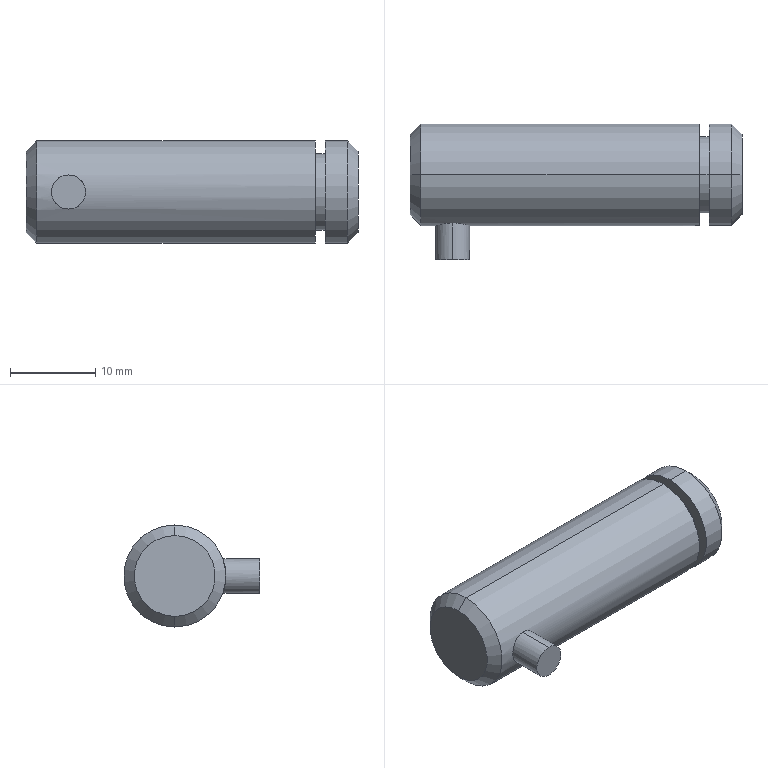Part | SolidWorks | features Revolution 2, Chamfer 1 | 1 solid | 17 faces | box 39 x 16 x 12 mm | volume 4350 mm3 | cylinder 8 | plane 5 | cone 4 | commonest cylinder face diameters 12 x4 4 x2 9 x2
STEP:
#1=CARTESIAN_POINT('',(19.5,0.,-4.75));
#2=VERTEX_POINT('',#1);
#3=CARTESIAN_POINT('',(19.5,0.,4.75));
#4=VERTEX_POINT('',#3);
#5=CARTESIAN_POINT('',(19.5,0.,0.));
#6=DIRECTION('',(1.,0.,0.));
#7=DIRECTION('',(0.,0.,-1.));
#8=AXIS2_PLACEMENT_3D('',#5,#6,#7);
#9=CIRCLE('',#8,4.75);
#10=EDGE_CURVE('',#2,#4,#9,.T.);
#11=ORIENTED_EDGE('',*,*,#10,.F.);
#12=CARTESIAN_POINT('',(18.25,0.,-6.));
#13=VERTEX_POINT('',#12);
#14=CARTESIAN_POINT('',(18.25,0.,-6.));
#15=DIRECTION('',(-0.7071,0.,-0.7071));
#16=VECTOR('',#15,1000.);
#17=LINE('',#14,#16);
#18=EDGE_CURVE('',#2,#13,#17,.T.);
#19=ORIENTED_EDGE('',*,*,#18,.T.);
#20=CARTESIAN_POINT('',(18.25,0.,6.));
#21=VERTEX_POINT('',#20);
#22=CARTESIAN_POINT('',(18.25,0.,0.));
#23=DIRECTION('',(-1.,0.,0.));
#24=DIRECTION('',(0.,0.,-1.));
#25=AXIS2_PLACEMENT_3D('',#22,#23,#24);
#26=CIRCLE('',#25,6.);
#27=EDGE_CURVE('',#21,#13,#26,.T.);
#28=ORIENTED_EDGE('',*,*,#27,.F.);
#29=CARTESIAN_POINT('',(18.25,0.,6.));
#30=DIRECTION('',(-0.7071,0.,0.7071));
#31=VECTOR('',#30,1000.);
#32=LINE('',#29,#31);
#33=EDGE_CURVE('',#4,#21,#32,.T.);
#34=ORIENTED_EDGE('',*,*,#33,.F.);
#35=EDGE_LOOP('',(#11,#19,#28,#34));
#36=FACE_OUTER_BOUND('',#35,.T.);
#37=CARTESIAN_POINT('',(18.25,0.,0.));
#38=DIRECTION('',(-1.,0.,0.));
#39=DIRECTION('',(0.,0.,1.));
#40=AXIS2_PLACEMENT_3D('',#37,#38,#39);
#41=CONICAL_SURFACE('',#40,6.,0.7854);
#42=ADVANCED_FACE('',(#36),#41,.T.);
#43=CARTESIAN_POINT('',(-19.5,0.,4.75));
#44=VERTEX_POINT('',#43);
#45=CARTESIAN_POINT('',(-19.5,0.,-4.75));
#46=VERTEX_POINT('',#45);
#47=CARTESIAN_POINT('',(-19.5,0.,0.));
#48=DIRECTION('',(-1.,0.,0.));
#49=DIRECTION('',(0.,0.,1.));
#50=AXIS2_PLACEMENT_3D('',#47,#48,#49);
#51=CIRCLE('',#50,4.75);
#52=EDGE_CURVE('',#44,#46,#51,.T.);
#53=ORIENTED_EDGE('',*,*,#52,.F.);
#54=CARTESIAN_POINT('',(-18.25,0.,6.));
#55=VERTEX_POINT('',#54);
#56=CARTESIAN_POINT('',(-19.5,0.,4.75));
#57=DIRECTION('',(0.7071,0.,0.7071));
#58=VECTOR('',#57,1000.);
#59=LINE('',#56,#58);
#60=EDGE_CURVE('',#44,#55,#59,.T.);
#61=ORIENTED_EDGE('',*,*,#60,.T.);
#62=CARTESIAN_POINT('',(-18.25,0.,-6.));
#63=VERTEX_POINT('',#62);
#64=CARTESIAN_POINT('',(-18.25,0.,0.));
#65=DIRECTION('',(1.,0.,0.));
#66=DIRECTION('',(0.,0.,1.));
#67=AXIS2_PLACEMENT_3D('',#64,#65,#66);
#68=CIRCLE('',#67,6.);
#69=EDGE_CURVE('',#63,#55,#68,.T.);
#70=ORIENTED_EDGE('',*,*,#69,.F.);
#71=CARTESIAN_POINT('',(-19.5,0.,-4.75));
#72=DIRECTION('',(0.7071,0.,-0.7071));
#73=VECTOR('',#72,1000.);
#74=LINE('',#71,#73);
#75=EDGE_CURVE('',#46,#63,#74,.T.);
#76=ORIENTED_EDGE('',*,*,#75,.F.);
#77=EDGE_LOOP('',(#53,#61,#70,#76));
#78=FACE_OUTER_BOUND('',#77,.T.);
#79=CARTESIAN_POINT('',(-19.5,0.,0.));
#80=DIRECTION('',(1.,0.,0.));
#81=DIRECTION('',(0.,0.,-1.));
#82=AXIS2_PLACEMENT_3D('',#79,#80,#81);
#83=CONICAL_SURFACE('',#82,4.75,0.7854);
#84=ADVANCED_FACE('',(#78),#83,.T.);
#85=CARTESIAN_POINT('',(-14.5,-5.657,-2.));
#86=VERTEX_POINT('',#85);
#87=CARTESIAN_POINT('',(-14.5,-5.657,2.));
#88=VERTEX_POINT('',#87);
#89=CARTESIAN_POINT('',(-14.5,-5.657,-2.));
#90=CARTESIAN_POINT('',(-14.367,-5.657,-2.));
#91=CARTESIAN_POINT('',(-14.236,-5.662,-1.987));
#92=CARTESIAN_POINT('',(-13.979,-5.679,-1.935));
#93=CARTESIAN_POINT('',(-13.852,-5.693,-1.897));
#94=CARTESIAN_POINT('',(-13.61,-5.725,-1.796));
#95=CARTESIAN_POINT('',(-13.495,-5.744,-1.734));
#96=CARTESIAN_POINT('',(-13.279,-5.786,-1.589));
#97=CARTESIAN_POINT('',(-13.177,-5.809,-1.506));
#98=CARTESIAN_POINT('',(-12.902,-5.875,-1.231));
#99=CARTESIAN_POINT('',(-12.754,-5.919,-1.009));
#100=CARTESIAN_POINT('',(-12.604,-5.966,-0.6487));
#101=CARTESIAN_POINT('',(-12.565,-5.979,-0.5216));
#102=CARTESIAN_POINT('',(-12.513,-5.996,-0.2629));
#103=CARTESIAN_POINT('',(-12.5,-6.,-0.1325));
#104=CARTESIAN_POINT('',(-12.5,-6.,0.1306));
#105=CARTESIAN_POINT('',(-12.513,-5.996,0.2642));
#106=CARTESIAN_POINT('',(-12.565,-5.979,0.5216));
#107=CARTESIAN_POINT('',(-12.603,-5.966,0.6468));
#108=CARTESIAN_POINT('',(-12.704,-5.935,0.8903));
#109=CARTESIAN_POINT('',(-12.766,-5.916,1.006));
#110=CARTESIAN_POINT('',(-12.911,-5.875,1.221));
#111=CARTESIAN_POINT('',(-12.995,-5.853,1.323));
#112=CARTESIAN_POINT('',(-13.179,-5.808,1.507));
#113=CARTESIAN_POINT('',(-13.279,-5.786,1.589));
#114=CARTESIAN_POINT('',(-13.495,-5.744,1.734));
#115=CARTESIAN_POINT('',(-13.612,-5.725,1.797));
#116=CARTESIAN_POINT('',(-13.853,-5.693,1.897));
#117=CARTESIAN_POINT('',(-13.977,-5.679,1.935));
#118=CARTESIAN_POINT('',(-14.236,-5.662,1.987));
#119=CARTESIAN_POINT('',(-14.369,-5.657,2.));
#120=CARTESIAN_POINT('',(-14.5,-5.657,2.));
#121=B_SPLINE_CURVE_WITH_KNOTS('',3,(#89,#90,#91,#92,#93,#94,#95,#96,#97,#98,#99,#100,#101,#102,#103,#104,#105,#106,#107,#108,#109,#110,#111,#112,#113,#114,#115,#116,#117,#118,#119,#120),.UNSPECIFIED.,.F.,.F.,(4,2,2,2,2,2,2,2,2,2,2,2,2,2,2,4),(0.,0.0003936,0.0007873,0.001181,0.001575,0.002362,0.002755,0.003149,0.003543,0.003936,0.00433,0.004724,0.005117,0.005511,0.005905,0.006298),.UNSPECIFIED.);
#122=EDGE_CURVE('',#86,#88,#121,.T.);
#123=ORIENTED_EDGE('',*,*,#122,.T.);
#124=CARTESIAN_POINT('',(-14.5,-10.,2.));
#125=VERTEX_POINT('',#124);
#126=CARTESIAN_POINT('',(-14.5,-5.657,2.));
#127=DIRECTION('',(0.,-1.,0.));
#128=VECTOR('',#127,1000.);
#129=LINE('',#126,#128);
#130=EDGE_CURVE('',#88,#125,#129,.T.);
#131=ORIENTED_EDGE('',*,*,#130,.T.);
#132=CARTESIAN_POINT('',(-14.5,-10.,-2.));
#133=VERTEX_POINT('',#132);
#134=CARTESIAN_POINT('',(-14.5,-10.,0.));
#135=DIRECTION('',(0.,-1.,0.));
#136=DIRECTION('',(0.,0.,-1.));
#137=AXIS2_PLACEMENT_3D('',#134,#135,#136);
#138=CIRCLE('',#137,2.);
#139=EDGE_CURVE('',#133,#125,#138,.T.);
#140=ORIENTED_EDGE('',*,*,#139,.F.);
#141=CARTESIAN_POINT('',(-14.5,-5.657,-2.));
#142=DIRECTION('',(0.,-1.,0.));
#143=VECTOR('',#142,1000.);
#144=LINE('',#141,#143);
#145=EDGE_CURVE('',#86,#133,#144,.T.);
#146=ORIENTED_EDGE('',*,*,#145,.F.);
#147=EDGE_LOOP('',(#123,#131,#140,#146));
#148=FACE_OUTER_BOUND('',#147,.T.);
#149=CARTESIAN_POINT('',(-14.5,-5.657,0.));
#150=DIRECTION('',(0.,-1.,0.));
#151=DIRECTION('',(0.,0.,-1.));
#152=AXIS2_PLACEMENT_3D('',#149,#150,#151);
#153=CYLINDRICAL_SURFACE('',#152,2.);
#154=ADVANCED_FACE('',(#148),#153,.T.);
#155=CARTESIAN_POINT('',(15.65,0.,4.5));
#156=VERTEX_POINT('',#155);
#157=CARTESIAN_POINT('',(15.65,0.,-4.5));
#158=VERTEX_POINT('',#157);
#159=CARTESIAN_POINT('',(15.65,0.,0.));
#160=DIRECTION('',(-1.,0.,0.));
#161=DIRECTION('',(0.,0.,1.));
#162=AXIS2_PLACEMENT_3D('',#159,#160,#161);
#163=CIRCLE('',#162,4.5);
#164=EDGE_CURVE('',#156,#158,#163,.T.);
#165=ORIENTED_EDGE('',*,*,#164,.T.);
#166=CARTESIAN_POINT('',(14.5,0.,-4.5));
#167=VERTEX_POINT('',#166);
#168=CARTESIAN_POINT('',(19.5,0.,-4.5));
#169=DIRECTION('',(-1.,0.,0.));
#170=VECTOR('',#169,1000.);
#171=LINE('',#168,#170);
#172=EDGE_CURVE('',#158,#167,#171,.T.);
#173=ORIENTED_EDGE('',*,*,#172,.T.);
#174=CARTESIAN_POINT('',(14.5,0.,4.5));
#175=VERTEX_POINT('',#174);
#176=CARTESIAN_POINT('',(14.5,0.,0.));
#177=DIRECTION('',(-1.,0.,0.));
#178=DIRECTION('',(0.,0.,1.));
#179=AXIS2_PLACEMENT_3D('',#176,#177,#178);
#180=CIRCLE('',#179,4.5);
#181=EDGE_CURVE('',#175,#167,#180,.T.);
#182=ORIENTED_EDGE('',*,*,#181,.F.);
#183=CARTESIAN_POINT('',(19.5,0.,4.5));
#184=DIRECTION('',(-1.,0.,0.));
#185=VECTOR('',#184,1000.);
#186=LINE('',#183,#185);
#187=EDGE_CURVE('',#156,#175,#186,.T.);
#188=ORIENTED_EDGE('',*,*,#187,.F.);
#189=EDGE_LOOP('',(#165,#173,#182,#188));
#190=FACE_OUTER_BOUND('',#189,.T.);
#191=CARTESIAN_POINT('',(19.5,0.,0.));
#192=DIRECTION('',(-1.,0.,0.));
#193=DIRECTION('',(0.,0.,1.));
#194=AXIS2_PLACEMENT_3D('',#191,#192,#193);
#195=CYLINDRICAL_SURFACE('',#194,4.5);
#196=ADVANCED_FACE('',(#190),#195,.T.);
#197=CARTESIAN_POINT('',(14.5,0.,6.));
#198=VERTEX_POINT('',#197);
#199=CARTESIAN_POINT('',(14.5,0.,-6.));
#200=VERTEX_POINT('',#199);
#201=CARTESIAN_POINT('',(14.5,0.,0.));
#202=DIRECTION('',(-1.,0.,0.));
#203=DIRECTION('',(0.,0.,1.));
#204=AXIS2_PLACEMENT_3D('',#201,#202,#203);
#205=CIRCLE('',#204,6.);
#206=EDGE_CURVE('',#198,#200,#205,.T.);
#207=ORIENTED_EDGE('',*,*,#206,.T.);
#208=CARTESIAN_POINT('',(19.5,0.,-6.));
#209=DIRECTION('',(-1.,0.,0.));
#210=VECTOR('',#209,1000.);
#211=LINE('',#208,#210);
#212=EDGE_CURVE('',#200,#63,#211,.T.);
#213=ORIENTED_EDGE('',*,*,#212,.T.);
#214=ORIENTED_EDGE('',*,*,#69,.T.);
#215=CARTESIAN_POINT('',(19.5,0.,6.));
#216=DIRECTION('',(-1.,0.,0.));
#217=VECTOR('',#216,1000.);
#218=LINE('',#215,#217);
#219=EDGE_CURVE('',#198,#55,#218,.T.);
#220=ORIENTED_EDGE('',*,*,#219,.F.);
#221=EDGE_LOOP('',(#207,#213,#214,#220));
#222=FACE_OUTER_BOUND('',#221,.T.);
#223=CARTESIAN_POINT('',(19.5,0.,0.));
#224=DIRECTION('',(-1.,0.,0.));
#225=DIRECTION('',(0.,0.,1.));
#226=AXIS2_PLACEMENT_3D('',#223,#224,#225);
#227=CYLINDRICAL_SURFACE('',#226,6.);
#228=ADVANCED_FACE('',(#222),#227,.T.);
#229=ORIENTED_EDGE('',*,*,#27,.T.);
#230=CARTESIAN_POINT('',(15.65,0.,-6.));
#231=VERTEX_POINT('',#230);
#232=CARTESIAN_POINT('',(19.5,0.,-6.));
#233=DIRECTION('',(-1.,0.,0.));
#234=VECTOR('',#233,1000.);
#235=LINE('',#232,#234);
#236=EDGE_CURVE('',#13,#231,#235,.T.);
#237=ORIENTED_EDGE('',*,*,#236,.T.);
#238=CARTESIAN_POINT('',(15.65,0.,6.));
#239=VERTEX_POINT('',#238);
#240=CARTESIAN_POINT('',(15.65,0.,0.));
#241=DIRECTION('',(-1.,0.,0.));
#242=DIRECTION('',(0.,0.,1.));
#243=AXIS2_PLACEMENT_3D('',#240,#241,#242);
#244=CIRCLE('',#243,6.);
#245=EDGE_CURVE('',#239,#231,#244,.T.);
#246=ORIENTED_EDGE('',*,*,#245,.F.);
#247=CARTESIAN_POINT('',(19.5,0.,6.));
#248=DIRECTION('',(-1.,0.,0.));
#249=VECTOR('',#248,1000.);
#250=LINE('',#247,#249);
#251=EDGE_CURVE('',#21,#239,#250,.T.);
#252=ORIENTED_EDGE('',*,*,#251,.F.);
#253=EDGE_LOOP('',(#229,#237,#246,#252));
#254=FACE_OUTER_BOUND('',#253,.T.);
#255=CARTESIAN_POINT('',(19.5,0.,0.));
#256=DIRECTION('',(-1.,0.,0.));
#257=DIRECTION('',(0.,0.,1.));
#258=AXIS2_PLACEMENT_3D('',#255,#256,#257);
#259=CYLINDRICAL_SURFACE('',#258,6.);
#260=ADVANCED_FACE('',(#254),#259,.T.);
#261=ORIENTED_EDGE('',*,*,#236,.F.);
#262=CARTESIAN_POINT('',(18.25,0.,0.));
#263=DIRECTION('',(-1.,0.,0.));
#264=DIRECTION('',(0.,0.,-1.));
#265=AXIS2_PLACEMENT_3D('',#262,#263,#264);
#266=CIRCLE('',#265,6.);
#267=EDGE_CURVE('',#13,#21,#266,.T.);
#268=ORIENTED_EDGE('',*,*,#267,.T.);
#269=ORIENTED_EDGE('',*,*,#251,.T.);
#270=CARTESIAN_POINT('',(15.65,0.,0.));
#271=DIRECTION('',(-1.,0.,0.));
#272=DIRECTION('',(0.,0.,1.));
#273=AXIS2_PLACEMENT_3D('',#270,#271,#272);
#274=CIRCLE('',#273,6.);
#275=EDGE_CURVE('',#231,#239,#274,.T.);
#276=ORIENTED_EDGE('',*,*,#275,.F.);
#277=EDGE_LOOP('',(#261,#268,#269,#276));
#278=FACE_OUTER_BOUND('',#277,.T.);
#279=CARTESIAN_POINT('',(19.5,0.,0.));
#280=DIRECTION('',(-1.,0.,0.));
#281=DIRECTION('',(0.,0.,1.));
#282=AXIS2_PLACEMENT_3D('',#279,#280,#281);
#283=CYLINDRICAL_SURFACE('',#282,6.);
#284=ADVANCED_FACE('',(#278),#283,.T.);
#285=CARTESIAN_POINT('',(19.5,0.,0.));
#286=DIRECTION('',(1.,0.,0.));
#287=DIRECTION('',(0.,0.,-1.));
#288=AXIS2_PLACEMENT_3D('',#285,#286,#287);
#289=CIRCLE('',#288,4.75);
#290=EDGE_CURVE('',#4,#2,#289,.T.);
#291=ORIENTED_EDGE('',*,*,#290,.T.);
#292=ORIENTED_EDGE('',*,*,#10,.T.);
#293=EDGE_LOOP('',(#291,#292));
#294=FACE_OUTER_BOUND('',#293,.T.);
#295=CARTESIAN_POINT('',(19.5,6.,0.));
#296=DIRECTION('',(1.,0.,0.));
#297=DIRECTION('',(0.,0.,-1.));
#298=AXIS2_PLACEMENT_3D('',#295,#296,#297);
#299=PLANE('',#298);
#300=ADVANCED_FACE('',(#294),#299,.T.);
#301=CARTESIAN_POINT('',(-19.5,0.,0.));
#302=DIRECTION('',(-1.,0.,0.));
#303=DIRECTION('',(0.,0.,1.));
#304=AXIS2_PLACEMENT_3D('',#301,#302,#303);
#305=CIRCLE('',#304,4.75);
#306=EDGE_CURVE('',#46,#44,#305,.T.);
#307=ORIENTED_EDGE('',*,*,#306,.T.);
#308=ORIENTED_EDGE('',*,*,#52,.T.);
#309=EDGE_LOOP('',(#307,#308));
#310=FACE_OUTER_BOUND('',#309,.T.);
#311=CARTESIAN_POINT('',(-19.5,0.,0.));
#312=DIRECTION('',(-1.,0.,0.));
#313=DIRECTION('',(0.,0.,1.));
#314=AXIS2_PLACEMENT_3D('',#311,#312,#313);
#315=PLANE('',#314);
#316=ADVANCED_FACE('',(#310),#315,.T.);
#317=ORIENTED_EDGE('',*,*,#212,.F.);
#318=CARTESIAN_POINT('',(14.5,0.,0.));
#319=DIRECTION('',(-1.,0.,0.));
#320=DIRECTION('',(0.,0.,1.));
#321=AXIS2_PLACEMENT_3D('',#318,#319,#320);
#322=CIRCLE('',#321,6.);
#323=EDGE_CURVE('',#200,#198,#322,.T.);
#324=ORIENTED_EDGE('',*,*,#323,.T.);
#325=ORIENTED_EDGE('',*,*,#219,.T.);
#326=CARTESIAN_POINT('',(-18.25,0.,0.));
#327=DIRECTION('',(1.,0.,0.));
#328=DIRECTION('',(0.,0.,1.));
#329=AXIS2_PLACEMENT_3D('',#326,#327,#328);
#330=CIRCLE('',#329,6.);
#331=EDGE_CURVE('',#55,#63,#330,.T.);
#332=ORIENTED_EDGE('',*,*,#331,.T.);
#333=EDGE_LOOP('',(#317,#324,#325,#332));
#334=FACE_OUTER_BOUND('',#333,.T.);
#335=ORIENTED_EDGE('',*,*,#122,.F.);
#336=CARTESIAN_POINT('',(-14.5,-5.657,2.));
#337=CARTESIAN_POINT('',(-14.762,-5.657,2.));
#338=CARTESIAN_POINT('',(-15.027,-5.676,1.947));
#339=CARTESIAN_POINT('',(-15.389,-5.725,1.796));
#340=CARTESIAN_POINT('',(-15.506,-5.745,1.734));
#341=CARTESIAN_POINT('',(-15.722,-5.786,1.589));
#342=CARTESIAN_POINT('',(-15.822,-5.809,1.507));
#343=CARTESIAN_POINT('',(-16.099,-5.876,1.23));
#344=CARTESIAN_POINT('',(-16.245,-5.919,1.011));
#345=CARTESIAN_POINT('',(-16.397,-5.966,0.6467));
#346=CARTESIAN_POINT('',(-16.435,-5.979,0.5217));
#347=CARTESIAN_POINT('',(-16.487,-5.996,0.2649));
#348=CARTESIAN_POINT('',(-16.5,-6.,0.1315));
#349=CARTESIAN_POINT('',(-16.5,-6.,-0.1321));
#350=CARTESIAN_POINT('',(-16.487,-5.996,-0.2626));
#351=CARTESIAN_POINT('',(-16.435,-5.979,-0.5211));
#352=CARTESIAN_POINT('',(-16.396,-5.966,-0.6484));
#353=CARTESIAN_POINT('',(-16.246,-5.919,-1.01));
#354=CARTESIAN_POINT('',(-16.097,-5.875,-1.231));
#355=CARTESIAN_POINT('',(-15.822,-5.809,-1.506));
#356=CARTESIAN_POINT('',(-15.72,-5.786,-1.59));
#357=CARTESIAN_POINT('',(-15.504,-5.744,-1.734));
#358=CARTESIAN_POINT('',(-15.39,-5.725,-1.796));
#359=CARTESIAN_POINT('',(-15.148,-5.693,-1.897));
#360=CARTESIAN_POINT('',(-15.021,-5.679,-1.935));
#361=CARTESIAN_POINT('',(-14.764,-5.662,-1.987));
#362=CARTESIAN_POINT('',(-14.633,-5.657,-2.));
#363=CARTESIAN_POINT('',(-14.5,-5.657,-2.));
#364=B_SPLINE_CURVE_WITH_KNOTS('',3,(#336,#337,#338,#339,#340,#341,#342,#343,#344,#345,#346,#347,#348,#349,#350,#351,#352,#353,#354,#355,#356,#357,#358,#359,#360,#361,#362,#363),.UNSPECIFIED.,.F.,.F.,(4,2,2,2,2,2,2,2,2,2,2,2,2,4),(0.006298,0.007085,0.007479,0.007872,0.008659,0.009053,0.009446,0.00984,0.01023,0.01102,0.01141,0.01181,0.0122,0.01259),.UNSPECIFIED.);
#365=EDGE_CURVE('',#88,#86,#364,.T.);
#366=ORIENTED_EDGE('',*,*,#365,.F.);
#367=EDGE_LOOP('',(#335,#366));
#368=FACE_BOUND('',#367,.T.);
#369=CARTESIAN_POINT('',(19.5,0.,0.));
#370=DIRECTION('',(-1.,0.,0.));
#371=DIRECTION('',(0.,0.,1.));
#372=AXIS2_PLACEMENT_3D('',#369,#370,#371);
#373=CYLINDRICAL_SURFACE('',#372,6.);
#374=ADVANCED_FACE('',(#334,#368),#373,.T.);
#375=ORIENTED_EDGE('',*,*,#181,.T.);
#376=CARTESIAN_POINT('',(14.5,0.,0.));
#377=DIRECTION('',(-1.,0.,0.));
#378=DIRECTION('',(0.,0.,1.));
#379=AXIS2_PLACEMENT_3D('',#376,#377,#378);
#380=CIRCLE('',#379,4.5);
#381=EDGE_CURVE('',#167,#175,#380,.T.);
#382=ORIENTED_EDGE('',*,*,#381,.T.);
#383=EDGE_LOOP('',(#375,#382));
#384=FACE_BOUND('',#383,.T.);
#385=ORIENTED_EDGE('',*,*,#206,.F.);
#386=ORIENTED_EDGE('',*,*,#323,.F.);
#387=EDGE_LOOP('',(#385,#386));
#388=FACE_OUTER_BOUND('',#387,.T.);
#389=CARTESIAN_POINT('',(14.5,6.,0.));
#390=DIRECTION('',(1.,0.,0.));
#391=DIRECTION('',(0.,0.,-1.));
#392=AXIS2_PLACEMENT_3D('',#389,#390,#391);
#393=PLANE('',#392);
#394=ADVANCED_FACE('',(#384,#388),#393,.T.);
#395=ORIENTED_EDGE('',*,*,#172,.F.);
#396=CARTESIAN_POINT('',(15.65,0.,0.));
#397=DIRECTION('',(-1.,0.,0.));
#398=DIRECTION('',(0.,0.,1.));
#399=AXIS2_PLACEMENT_3D('',#396,#397,#398);
#400=CIRCLE('',#399,4.5);
#401=EDGE_CURVE('',#158,#156,#400,.T.);
#402=ORIENTED_EDGE('',*,*,#401,.T.);
#403=ORIENTED_EDGE('',*,*,#187,.T.);
#404=ORIENTED_EDGE('',*,*,#381,.F.);
#405=EDGE_LOOP('',(#395,#402,#403,#404));
#406=FACE_OUTER_BOUND('',#405,.T.);
#407=CARTESIAN_POINT('',(19.5,0.,0.));
#408=DIRECTION('',(-1.,0.,0.));
#409=DIRECTION('',(0.,0.,1.));
#410=AXIS2_PLACEMENT_3D('',#407,#408,#409);
#411=CYLINDRICAL_SURFACE('',#410,4.5);
#412=ADVANCED_FACE('',(#406),#411,.T.);
#413=ORIENTED_EDGE('',*,*,#245,.T.);
#414=ORIENTED_EDGE('',*,*,#275,.T.);
#415=EDGE_LOOP('',(#413,#414));
#416=FACE_OUTER_BOUND('',#415,.T.);
#417=ORIENTED_EDGE('',*,*,#164,.F.);
#418=ORIENTED_EDGE('',*,*,#401,.F.);
#419=EDGE_LOOP('',(#417,#418));
#420=FACE_BOUND('',#419,.T.);
#421=CARTESIAN_POINT('',(15.65,4.5,0.));
#422=DIRECTION('',(-1.,0.,0.));
#423=DIRECTION('',(0.,0.,1.));
#424=AXIS2_PLACEMENT_3D('',#421,#422,#423);
#425=PLANE('',#424);
#426=ADVANCED_FACE('',(#416,#420),#425,.T.);
#427=ORIENTED_EDGE('',*,*,#139,.T.);
#428=CARTESIAN_POINT('',(-14.5,-10.,0.));
#429=DIRECTION('',(0.,-1.,0.));
#430=DIRECTION('',(0.,0.,-1.));
#431=AXIS2_PLACEMENT_3D('',#428,#429,#430);
#432=CIRCLE('',#431,2.);
#433=EDGE_CURVE('',#125,#133,#432,.T.);
#434=ORIENTED_EDGE('',*,*,#433,.T.);
#435=EDGE_LOOP('',(#427,#434));
#436=FACE_OUTER_BOUND('',#435,.T.);
#437=CARTESIAN_POINT('',(-14.5,-10.,0.));
#438=DIRECTION('',(0.,-1.,0.));
#439=DIRECTION('',(0.,0.,-1.));
#440=AXIS2_PLACEMENT_3D('',#437,#438,#439);
#441=PLANE('',#440);
#442=ADVANCED_FACE('',(#436),#441,.T.);
#443=ORIENTED_EDGE('',*,*,#130,.F.);
#444=ORIENTED_EDGE('',*,*,#365,.T.);
#445=ORIENTED_EDGE('',*,*,#145,.T.);
#446=ORIENTED_EDGE('',*,*,#433,.F.);
#447=EDGE_LOOP('',(#443,#444,#445,#446));
#448=FACE_OUTER_BOUND('',#447,.T.);
#449=CARTESIAN_POINT('',(-14.5,-5.657,0.));
#450=DIRECTION('',(0.,-1.,0.));
#451=DIRECTION('',(0.,0.,-1.));
#452=AXIS2_PLACEMENT_3D('',#449,#450,#451);
#453=CYLINDRICAL_SURFACE('',#452,2.);
#454=ADVANCED_FACE('',(#448),#453,.T.);
#455=ORIENTED_EDGE('',*,*,#60,.F.);
#456=ORIENTED_EDGE('',*,*,#306,.F.);
#457=ORIENTED_EDGE('',*,*,#75,.T.);
#458=ORIENTED_EDGE('',*,*,#331,.F.);
#459=EDGE_LOOP('',(#455,#456,#457,#458));
#460=FACE_OUTER_BOUND('',#459,.T.);
#461=CARTESIAN_POINT('',(-19.5,0.,0.));
#462=DIRECTION('',(1.,0.,0.));
#463=DIRECTION('',(0.,0.,-1.));
#464=AXIS2_PLACEMENT_3D('',#461,#462,#463);
#465=CONICAL_SURFACE('',#464,4.75,0.7854);
#466=ADVANCED_FACE('',(#460),#465,.T.);
#467=ORIENTED_EDGE('',*,*,#18,.F.);
#468=ORIENTED_EDGE('',*,*,#290,.F.);
#469=ORIENTED_EDGE('',*,*,#33,.T.);
#470=ORIENTED_EDGE('',*,*,#267,.F.);
#471=EDGE_LOOP('',(#467,#468,#469,#470));
#472=FACE_OUTER_BOUND('',#471,.T.);
#473=CARTESIAN_POINT('',(18.25,0.,0.));
#474=DIRECTION('',(-1.,0.,0.));
#475=DIRECTION('',(0.,0.,1.));
#476=AXIS2_PLACEMENT_3D('',#473,#474,#475);
#477=CONICAL_SURFACE('',#476,6.,0.7854);
#478=ADVANCED_FACE('',(#472),#477,.T.);
#479=CLOSED_SHELL('',(#42,#84,#154,#196,#228,#260,#284,#300,#316,#374,#394,#412,#426,#442,#454,#466,#478));
#480=MANIFOLD_SOLID_BREP('',#479);
#481=CARTESIAN_POINT('',(0.,0.,0.));
#482=DIRECTION('',(0.,0.,1.));
#483=DIRECTION('',(1.,0.,0.));
#484=AXIS2_PLACEMENT_3D('',#481,#482,#483);
#485=(LENGTH_UNIT()NAMED_UNIT(*)SI_UNIT(.MILLI.,.METRE.));
#486=UNCERTAINTY_MEASURE_WITH_UNIT(LENGTH_MEASURE(0.00001),#485,'','');
#487=(NAMED_UNIT(*)PLANE_ANGLE_UNIT()SI_UNIT($,.RADIAN.));
#488=(NAMED_UNIT(*)SI_UNIT($,.STERADIAN.)SOLID_ANGLE_UNIT());
#489=(GEOMETRIC_REPRESENTATION_CONTEXT(3)GLOBAL_UNCERTAINTY_ASSIGNED_CONTEXT((#486))GLOBAL_UNIT_ASSIGNED_CONTEXT((#485,#487,#488))REPRESENTATION_CONTEXT('',''));
#490=ADVANCED_BREP_SHAPE_REPRESENTATION('',(#480,#484),#489);